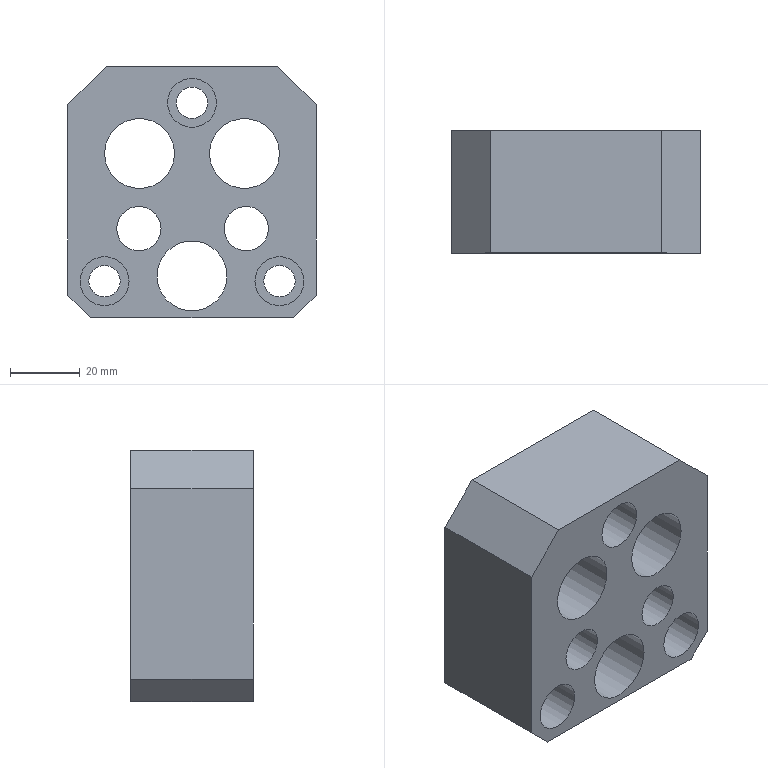Part | STEP file | 1_id594_x_t | 1 solid | 28 faces | box 71 x 35 x 72 mm | volume 118326 mm3 | plane 15 | cylinder 13 | commonest cylinder face diameters 9 x3 14 x3 20 x3 12.7 x2 16.875 x2